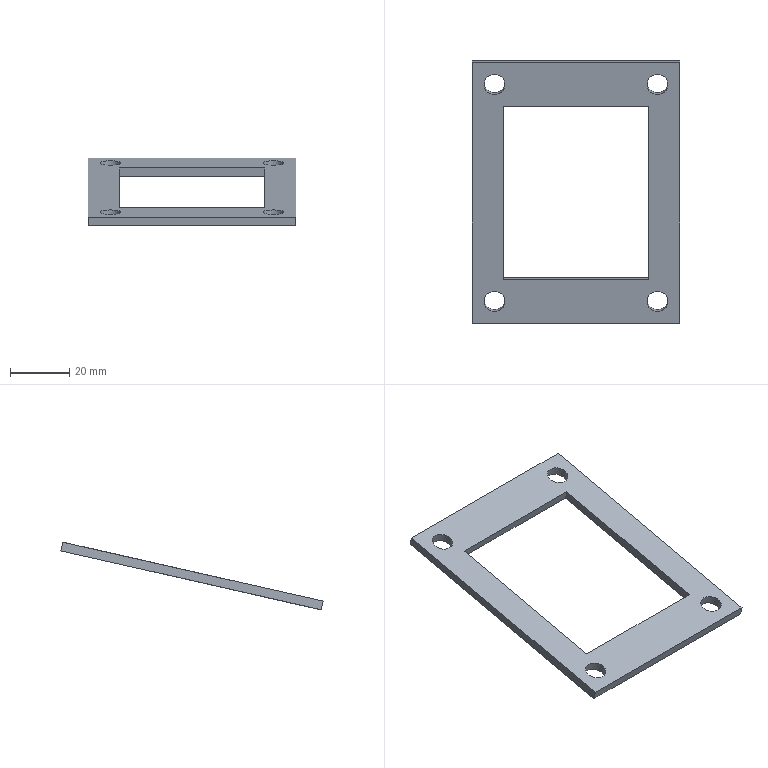Part | NX | features DATUM_CSYS 38, SIMPLE HOLE 38, SKETCH 37, EXTRACT_DATUM_AXIS 32, EXTRACT_FACE 26, HOLE PACKAGE 25, EXTRUDE 21, EXTRACT_DATUM_PLANE 14, Instance Feature 10, DRAFT 8, EXTRACT_STRING 8, BLEND 5, FSET 4, Mirror Feature 4, OFFSET_REGION 4, REPLACE_FACE 3, CPROJ 2, Pattern Feature 2, DATUM_PLANE 1, TRIM BODY 1 | 1 solid | 14 faces | box 70 x 88.433 x 22.841 mm | volume 9618 mm3 | plane 10 | cylinder 4 | commonest cylinder face diameters 7 x4
STEP:
#1=CARTESIAN_POINT('',(-35.,81.613,102.603));
#2=VERTEX_POINT('',#1);
#3=CARTESIAN_POINT('',(-35.,-6.156,82.688));
#4=VERTEX_POINT('',#3);
#5=CARTESIAN_POINT('',(-35.,81.613,102.603));
#6=DIRECTION('',(0.,-0.9752,-0.2213));
#7=VECTOR('',#6,1000.);
#8=LINE('',#5,#7);
#9=EDGE_CURVE('',#2,#4,#8,.T.);
#10=ORIENTED_EDGE('',*,*,#9,.F.);
#11=CARTESIAN_POINT('',(35.,81.613,102.603));
#12=VERTEX_POINT('',#11);
#13=CARTESIAN_POINT('',(35.,81.613,102.603));
#14=DIRECTION('',(-1.,0.,0.));
#15=VECTOR('',#14,1000.);
#16=LINE('',#13,#15);
#17=EDGE_CURVE('',#12,#2,#16,.T.);
#18=ORIENTED_EDGE('',*,*,#17,.F.);
#19=CARTESIAN_POINT('',(35.,-6.156,82.688));
#20=VERTEX_POINT('',#19);
#21=CARTESIAN_POINT('',(35.,-6.156,82.688));
#22=DIRECTION('',(0.,0.9752,0.2213));
#23=VECTOR('',#22,1000.);
#24=LINE('',#21,#23);
#25=EDGE_CURVE('',#20,#12,#24,.T.);
#26=ORIENTED_EDGE('',*,*,#25,.F.);
#27=CARTESIAN_POINT('',(-35.,-6.156,82.688));
#28=DIRECTION('',(1.,0.,0.));
#29=VECTOR('',#28,1000.);
#30=LINE('',#27,#29);
#31=EDGE_CURVE('',#4,#20,#30,.T.);
#32=ORIENTED_EDGE('',*,*,#31,.F.);
#33=EDGE_LOOP('',(#10,#18,#26,#32));
#34=FACE_BOUND('',#33,.T.);
#35=CARTESIAN_POINT('',(-27.5,4.572,85.122));
#36=VERTEX_POINT('',#35);
#37=CARTESIAN_POINT('',(-27.5,1.158,84.347));
#38=DIRECTION('',(0.,0.2213,-0.9752));
#39=DIRECTION('',(0.,0.9752,0.2213));
#40=AXIS2_PLACEMENT_3D('',#37,#38,#39);
#41=CIRCLE('',#40,3.5);
#42=EDGE_CURVE('',#36,#36,#41,.F.);
#43=ORIENTED_EDGE('',*,*,#42,.T.);
#44=EDGE_LOOP('',(#43));
#45=FACE_BOUND('',#44,.T.);
#46=CARTESIAN_POINT('',(27.5,4.572,85.122));
#47=VERTEX_POINT('',#46);
#48=CARTESIAN_POINT('',(27.5,1.158,84.347));
#49=DIRECTION('',(0.,0.2213,-0.9752));
#50=DIRECTION('',(0.,0.9752,0.2213));
#51=AXIS2_PLACEMENT_3D('',#48,#49,#50);
#52=CIRCLE('',#51,3.5);
#53=EDGE_CURVE('',#47,#47,#52,.T.);
#54=ORIENTED_EDGE('',*,*,#53,.F.);
#55=EDGE_LOOP('',(#54));
#56=FACE_BOUND('',#55,.T.);
#57=CARTESIAN_POINT('',(24.5,66.985,99.283));
#58=VERTEX_POINT('',#57);
#59=CARTESIAN_POINT('',(-24.5,66.985,99.283));
#60=VERTEX_POINT('',#59);
#61=CARTESIAN_POINT('',(-24.5,66.985,99.283));
#62=DIRECTION('',(-1.,0.,0.));
#63=VECTOR('',#62,1000.);
#64=LINE('',#61,#63);
#65=EDGE_CURVE('',#58,#60,#64,.T.);
#66=ORIENTED_EDGE('',*,*,#65,.T.);
#67=CARTESIAN_POINT('',(-24.5,8.472,86.007));
#68=VERTEX_POINT('',#67);
#69=CARTESIAN_POINT('',(-24.5,8.472,86.007));
#70=DIRECTION('',(0.,-0.9752,-0.2213));
#71=VECTOR('',#70,1000.);
#72=LINE('',#69,#71);
#73=EDGE_CURVE('',#60,#68,#72,.T.);
#74=ORIENTED_EDGE('',*,*,#73,.T.);
#75=CARTESIAN_POINT('',(24.5,8.472,86.007));
#76=VERTEX_POINT('',#75);
#77=CARTESIAN_POINT('',(24.5,8.472,86.007));
#78=DIRECTION('',(1.,0.,0.));
#79=VECTOR('',#78,1000.);
#80=LINE('',#77,#79);
#81=EDGE_CURVE('',#68,#76,#80,.T.);
#82=ORIENTED_EDGE('',*,*,#81,.T.);
#83=CARTESIAN_POINT('',(24.5,66.985,99.283));
#84=DIRECTION('',(0.,0.9752,0.2213));
#85=VECTOR('',#84,1000.);
#86=LINE('',#83,#85);
#87=EDGE_CURVE('',#76,#58,#86,.T.);
#88=ORIENTED_EDGE('',*,*,#87,.T.);
#89=EDGE_LOOP('',(#66,#74,#82,#88));
#90=FACE_BOUND('',#89,.T.);
#91=CARTESIAN_POINT('',(-27.5,77.712,101.717));
#92=VERTEX_POINT('',#91);
#93=CARTESIAN_POINT('',(-27.5,74.299,100.943));
#94=DIRECTION('',(0.,0.2213,-0.9752));
#95=DIRECTION('',(0.,0.9752,0.2213));
#96=AXIS2_PLACEMENT_3D('',#93,#94,#95);
#97=CIRCLE('',#96,3.5);
#98=EDGE_CURVE('',#92,#92,#97,.T.);
#99=ORIENTED_EDGE('',*,*,#98,.F.);
#100=EDGE_LOOP('',(#99));
#101=FACE_BOUND('',#100,.T.);
#102=CARTESIAN_POINT('',(27.5,77.712,101.717));
#103=VERTEX_POINT('',#102);
#104=CARTESIAN_POINT('',(27.5,74.299,100.943));
#105=DIRECTION('',(0.,0.2213,-0.9752));
#106=DIRECTION('',(0.,0.9752,0.2213));
#107=AXIS2_PLACEMENT_3D('',#104,#105,#106);
#108=CIRCLE('',#107,3.5);
#109=EDGE_CURVE('',#103,#103,#108,.F.);
#110=ORIENTED_EDGE('',*,*,#109,.T.);
#111=EDGE_LOOP('',(#110));
#112=FACE_BOUND('',#111,.T.);
#113=CARTESIAN_POINT('',(0.,37.729,92.645));
#114=DIRECTION('',(0.,0.2213,-0.9752));
#115=DIRECTION('',(0.,0.9752,0.2213));
#116=AXIS2_PLACEMENT_3D('',#113,#114,#115);
#117=PLANE('',#116);
#118=ADVANCED_FACE('',(#34,#45,#56,#90,#101,#112),#117,.T.);
#119=CARTESIAN_POINT('',(27.5,77.049,104.643));
#120=VERTEX_POINT('',#119);
#121=CARTESIAN_POINT('',(27.5,73.635,103.869));
#122=DIRECTION('',(0.,0.2213,-0.9752));
#123=DIRECTION('',(0.,0.9752,0.2213));
#124=AXIS2_PLACEMENT_3D('',#121,#122,#123);
#125=CIRCLE('',#124,3.5);
#126=EDGE_CURVE('',#120,#120,#125,.T.);
#127=ORIENTED_EDGE('',*,*,#126,.F.);
#128=EDGE_LOOP('',(#127));
#129=FACE_BOUND('',#128,.T.);
#130=ORIENTED_EDGE('',*,*,#109,.F.);
#131=EDGE_LOOP('',(#130));
#132=FACE_BOUND('',#131,.T.);
#133=CARTESIAN_POINT('',(27.5,73.414,104.844));
#134=DIRECTION('',(0.,0.2213,-0.9752));
#135=DIRECTION('',(0.,0.9752,0.2213));
#136=AXIS2_PLACEMENT_3D('',#133,#134,#135);
#137=CYLINDRICAL_SURFACE('',#136,3.5);
#138=ADVANCED_FACE('',(#129,#132),#137,.F.);
#139=CARTESIAN_POINT('',(-27.5,77.049,104.643));
#140=VERTEX_POINT('',#139);
#141=CARTESIAN_POINT('',(-27.5,73.635,103.869));
#142=DIRECTION('',(0.,0.2213,-0.9752));
#143=DIRECTION('',(0.,0.9752,0.2213));
#144=AXIS2_PLACEMENT_3D('',#141,#142,#143);
#145=CIRCLE('',#144,3.5);
#146=EDGE_CURVE('',#140,#140,#145,.F.);
#147=ORIENTED_EDGE('',*,*,#146,.T.);
#148=EDGE_LOOP('',(#147));
#149=FACE_BOUND('',#148,.T.);
#150=ORIENTED_EDGE('',*,*,#98,.T.);
#151=EDGE_LOOP('',(#150));
#152=FACE_BOUND('',#151,.T.);
#153=CARTESIAN_POINT('',(-27.5,73.414,104.844));
#154=DIRECTION('',(0.,0.2213,-0.9752));
#155=DIRECTION('',(0.,0.9752,0.2213));
#156=AXIS2_PLACEMENT_3D('',#153,#154,#155);
#157=CYLINDRICAL_SURFACE('',#156,3.5);
#158=ADVANCED_FACE('',(#149,#152),#157,.F.);
#159=ORIENTED_EDGE('',*,*,#73,.F.);
#160=CARTESIAN_POINT('',(-24.5,66.321,102.209));
#161=VERTEX_POINT('',#160);
#162=CARTESIAN_POINT('',(-24.5,66.1,103.184));
#163=DIRECTION('',(0.,0.2213,-0.9752));
#164=VECTOR('',#163,1000.);
#165=LINE('',#162,#164);
#166=EDGE_CURVE('',#161,#60,#165,.T.);
#167=ORIENTED_EDGE('',*,*,#166,.F.);
#168=CARTESIAN_POINT('',(-24.5,7.809,88.932));
#169=VERTEX_POINT('',#168);
#170=CARTESIAN_POINT('',(-24.5,73.635,103.869));
#171=DIRECTION('',(0.,0.9752,0.2213));
#172=VECTOR('',#171,1000.);
#173=LINE('',#170,#172);
#174=EDGE_CURVE('',#169,#161,#173,.T.);
#175=ORIENTED_EDGE('',*,*,#174,.F.);
#176=CARTESIAN_POINT('',(-24.5,7.587,89.908));
#177=DIRECTION('',(0.,0.2213,-0.9752));
#178=VECTOR('',#177,1000.);
#179=LINE('',#176,#178);
#180=EDGE_CURVE('',#169,#68,#179,.T.);
#181=ORIENTED_EDGE('',*,*,#180,.T.);
#182=EDGE_LOOP('',(#159,#167,#175,#181));
#183=FACE_BOUND('',#182,.T.);
#184=CARTESIAN_POINT('',(-24.5,7.587,89.908));
#185=DIRECTION('',(-1.,0.,0.));
#186=DIRECTION('',(0.,0.,1.));
#187=AXIS2_PLACEMENT_3D('',#184,#185,#186);
#188=PLANE('',#187);
#189=ADVANCED_FACE('',(#183),#188,.F.);
#190=ORIENTED_EDGE('',*,*,#65,.F.);
#191=CARTESIAN_POINT('',(24.5,66.321,102.209));
#192=VERTEX_POINT('',#191);
#193=CARTESIAN_POINT('',(24.5,66.1,103.184));
#194=DIRECTION('',(0.,0.2213,-0.9752));
#195=VECTOR('',#194,1000.);
#196=LINE('',#193,#195);
#197=EDGE_CURVE('',#192,#58,#196,.T.);
#198=ORIENTED_EDGE('',*,*,#197,.F.);
#199=CARTESIAN_POINT('',(27.5,66.321,102.209));
#200=DIRECTION('',(1.,0.,0.));
#201=VECTOR('',#200,1000.);
#202=LINE('',#199,#201);
#203=EDGE_CURVE('',#161,#192,#202,.T.);
#204=ORIENTED_EDGE('',*,*,#203,.F.);
#205=ORIENTED_EDGE('',*,*,#166,.T.);
#206=EDGE_LOOP('',(#190,#198,#204,#205));
#207=FACE_BOUND('',#206,.T.);
#208=CARTESIAN_POINT('',(-24.5,66.1,103.184));
#209=DIRECTION('',(0.,0.9752,0.2213));
#210=DIRECTION('',(0.,-0.2213,0.9752));
#211=AXIS2_PLACEMENT_3D('',#208,#209,#210);
#212=PLANE('',#211);
#213=ADVANCED_FACE('',(#207),#212,.F.);
#214=ORIENTED_EDGE('',*,*,#87,.F.);
#215=CARTESIAN_POINT('',(24.5,7.809,88.932));
#216=VERTEX_POINT('',#215);
#217=CARTESIAN_POINT('',(24.5,7.587,89.908));
#218=DIRECTION('',(0.,0.2213,-0.9752));
#219=VECTOR('',#218,1000.);
#220=LINE('',#217,#219);
#221=EDGE_CURVE('',#216,#76,#220,.T.);
#222=ORIENTED_EDGE('',*,*,#221,.F.);
#223=CARTESIAN_POINT('',(24.5,73.635,103.869));
#224=DIRECTION('',(0.,-0.9752,-0.2213));
#225=VECTOR('',#224,1000.);
#226=LINE('',#223,#225);
#227=EDGE_CURVE('',#192,#216,#226,.T.);
#228=ORIENTED_EDGE('',*,*,#227,.F.);
#229=ORIENTED_EDGE('',*,*,#197,.T.);
#230=EDGE_LOOP('',(#214,#222,#228,#229));
#231=FACE_BOUND('',#230,.T.);
#232=CARTESIAN_POINT('',(24.5,66.1,103.184));
#233=DIRECTION('',(1.,0.,0.));
#234=DIRECTION('',(0.,0.,-1.));
#235=AXIS2_PLACEMENT_3D('',#232,#233,#234);
#236=PLANE('',#235);
#237=ADVANCED_FACE('',(#231),#236,.F.);
#238=CARTESIAN_POINT('',(-27.5,3.908,88.047));
#239=VERTEX_POINT('',#238);
#240=CARTESIAN_POINT('',(-27.5,0.4945,87.273));
#241=DIRECTION('',(0.,0.2213,-0.9752));
#242=DIRECTION('',(0.,0.9752,0.2213));
#243=AXIS2_PLACEMENT_3D('',#240,#241,#242);
#244=CIRCLE('',#243,3.5);
#245=EDGE_CURVE('',#239,#239,#244,.T.);
#246=ORIENTED_EDGE('',*,*,#245,.F.);
#247=EDGE_LOOP('',(#246));
#248=FACE_BOUND('',#247,.T.);
#249=ORIENTED_EDGE('',*,*,#42,.F.);
#250=EDGE_LOOP('',(#249));
#251=FACE_BOUND('',#250,.T.);
#252=CARTESIAN_POINT('',(-27.5,0.2732,88.248));
#253=DIRECTION('',(0.,0.2213,-0.9752));
#254=DIRECTION('',(0.,0.9752,0.2213));
#255=AXIS2_PLACEMENT_3D('',#252,#253,#254);
#256=CYLINDRICAL_SURFACE('',#255,3.5);
#257=ADVANCED_FACE('',(#248,#251),#256,.F.);
#258=CARTESIAN_POINT('',(27.5,3.908,88.047));
#259=VERTEX_POINT('',#258);
#260=CARTESIAN_POINT('',(27.5,0.4945,87.273));
#261=DIRECTION('',(0.,0.2213,-0.9752));
#262=DIRECTION('',(0.,0.9752,0.2213));
#263=AXIS2_PLACEMENT_3D('',#260,#261,#262);
#264=CIRCLE('',#263,3.5);
#265=EDGE_CURVE('',#259,#259,#264,.F.);
#266=ORIENTED_EDGE('',*,*,#265,.T.);
#267=EDGE_LOOP('',(#266));
#268=FACE_BOUND('',#267,.T.);
#269=ORIENTED_EDGE('',*,*,#53,.T.);
#270=EDGE_LOOP('',(#269));
#271=FACE_BOUND('',#270,.T.);
#272=CARTESIAN_POINT('',(27.5,0.2732,88.248));
#273=DIRECTION('',(0.,0.2213,-0.9752));
#274=DIRECTION('',(0.,0.9752,0.2213));
#275=AXIS2_PLACEMENT_3D('',#272,#273,#274);
#276=CYLINDRICAL_SURFACE('',#275,3.5);
#277=ADVANCED_FACE('',(#268,#271),#276,.F.);
#278=ORIENTED_EDGE('',*,*,#81,.F.);
#279=ORIENTED_EDGE('',*,*,#180,.F.);
#280=CARTESIAN_POINT('',(27.5,7.809,88.932));
#281=DIRECTION('',(-1.,0.,0.));
#282=VECTOR('',#281,1000.);
#283=LINE('',#280,#282);
#284=EDGE_CURVE('',#216,#169,#283,.T.);
#285=ORIENTED_EDGE('',*,*,#284,.F.);
#286=ORIENTED_EDGE('',*,*,#221,.T.);
#287=EDGE_LOOP('',(#278,#279,#285,#286));
#288=FACE_BOUND('',#287,.T.);
#289=CARTESIAN_POINT('',(24.5,7.587,89.908));
#290=DIRECTION('',(0.,-0.9752,-0.2213));
#291=DIRECTION('',(0.,0.2213,-0.9752));
#292=AXIS2_PLACEMENT_3D('',#289,#290,#291);
#293=PLANE('',#292);
#294=ADVANCED_FACE('',(#288),#293,.F.);
#295=ORIENTED_EDGE('',*,*,#9,.T.);
#296=CARTESIAN_POINT('',(-35.,-6.82,85.613));
#297=VERTEX_POINT('',#296);
#298=CARTESIAN_POINT('',(-35.,-7.041,86.588));
#299=DIRECTION('',(0.,0.2213,-0.9752));
#300=VECTOR('',#299,1000.);
#301=LINE('',#298,#300);
#302=EDGE_CURVE('',#297,#4,#301,.T.);
#303=ORIENTED_EDGE('',*,*,#302,.F.);
#304=CARTESIAN_POINT('',(-35.,80.949,105.528));
#305=VERTEX_POINT('',#304);
#306=CARTESIAN_POINT('',(-35.,73.635,103.869));
#307=DIRECTION('',(0.,-0.9752,-0.2213));
#308=VECTOR('',#307,1000.);
#309=LINE('',#306,#308);
#310=EDGE_CURVE('',#305,#297,#309,.T.);
#311=ORIENTED_EDGE('',*,*,#310,.F.);
#312=CARTESIAN_POINT('',(-35.,80.728,106.503));
#313=DIRECTION('',(0.,0.2213,-0.9752));
#314=VECTOR('',#313,1000.);
#315=LINE('',#312,#314);
#316=EDGE_CURVE('',#305,#2,#315,.T.);
#317=ORIENTED_EDGE('',*,*,#316,.T.);
#318=EDGE_LOOP('',(#295,#303,#311,#317));
#319=FACE_BOUND('',#318,.T.);
#320=CARTESIAN_POINT('',(-35.,80.728,106.503));
#321=DIRECTION('',(1.,0.,0.));
#322=DIRECTION('',(0.,0.,-1.));
#323=AXIS2_PLACEMENT_3D('',#320,#321,#322);
#324=PLANE('',#323);
#325=ADVANCED_FACE('',(#319),#324,.F.);
#326=ORIENTED_EDGE('',*,*,#31,.T.);
#327=CARTESIAN_POINT('',(35.,-6.82,85.613));
#328=VERTEX_POINT('',#327);
#329=CARTESIAN_POINT('',(35.,-7.041,86.588));
#330=DIRECTION('',(0.,0.2213,-0.9752));
#331=VECTOR('',#330,1000.);
#332=LINE('',#329,#331);
#333=EDGE_CURVE('',#328,#20,#332,.T.);
#334=ORIENTED_EDGE('',*,*,#333,.F.);
#335=CARTESIAN_POINT('',(27.5,-6.82,85.613));
#336=DIRECTION('',(1.,0.,0.));
#337=VECTOR('',#336,1000.);
#338=LINE('',#335,#337);
#339=EDGE_CURVE('',#297,#328,#338,.T.);
#340=ORIENTED_EDGE('',*,*,#339,.F.);
#341=ORIENTED_EDGE('',*,*,#302,.T.);
#342=EDGE_LOOP('',(#326,#334,#340,#341));
#343=FACE_BOUND('',#342,.T.);
#344=CARTESIAN_POINT('',(-35.,-7.041,86.588));
#345=DIRECTION('',(0.,0.9752,0.2213));
#346=DIRECTION('',(0.,-0.2213,0.9752));
#347=AXIS2_PLACEMENT_3D('',#344,#345,#346);
#348=PLANE('',#347);
#349=ADVANCED_FACE('',(#343),#348,.F.);
#350=ORIENTED_EDGE('',*,*,#25,.T.);
#351=CARTESIAN_POINT('',(35.,80.949,105.528));
#352=VERTEX_POINT('',#351);
#353=CARTESIAN_POINT('',(35.,80.728,106.503));
#354=DIRECTION('',(0.,0.2213,-0.9752));
#355=VECTOR('',#354,1000.);
#356=LINE('',#353,#355);
#357=EDGE_CURVE('',#352,#12,#356,.T.);
#358=ORIENTED_EDGE('',*,*,#357,.F.);
#359=CARTESIAN_POINT('',(35.,73.635,103.869));
#360=DIRECTION('',(0.,0.9752,0.2213));
#361=VECTOR('',#360,1000.);
#362=LINE('',#359,#361);
#363=EDGE_CURVE('',#328,#352,#362,.T.);
#364=ORIENTED_EDGE('',*,*,#363,.F.);
#365=ORIENTED_EDGE('',*,*,#333,.T.);
#366=EDGE_LOOP('',(#350,#358,#364,#365));
#367=FACE_BOUND('',#366,.T.);
#368=CARTESIAN_POINT('',(35.,-7.041,86.588));
#369=DIRECTION('',(-1.,0.,0.));
#370=DIRECTION('',(0.,0.,1.));
#371=AXIS2_PLACEMENT_3D('',#368,#369,#370);
#372=PLANE('',#371);
#373=ADVANCED_FACE('',(#367),#372,.F.);
#374=ORIENTED_EDGE('',*,*,#17,.T.);
#375=ORIENTED_EDGE('',*,*,#316,.F.);
#376=CARTESIAN_POINT('',(27.5,80.949,105.528));
#377=DIRECTION('',(-1.,0.,0.));
#378=VECTOR('',#377,1000.);
#379=LINE('',#376,#378);
#380=EDGE_CURVE('',#352,#305,#379,.T.);
#381=ORIENTED_EDGE('',*,*,#380,.F.);
#382=ORIENTED_EDGE('',*,*,#357,.T.);
#383=EDGE_LOOP('',(#374,#375,#381,#382));
#384=FACE_BOUND('',#383,.T.);
#385=CARTESIAN_POINT('',(35.,80.728,106.503));
#386=DIRECTION('',(0.,-0.9752,-0.2213));
#387=DIRECTION('',(0.,0.2213,-0.9752));
#388=AXIS2_PLACEMENT_3D('',#385,#386,#387);
#389=PLANE('',#388);
#390=ADVANCED_FACE('',(#384),#389,.F.);
#391=ORIENTED_EDGE('',*,*,#310,.T.);
#392=ORIENTED_EDGE('',*,*,#339,.T.);
#393=ORIENTED_EDGE('',*,*,#363,.T.);
#394=ORIENTED_EDGE('',*,*,#380,.T.);
#395=EDGE_LOOP('',(#391,#392,#393,#394));
#396=FACE_BOUND('',#395,.T.);
#397=ORIENTED_EDGE('',*,*,#126,.T.);
#398=EDGE_LOOP('',(#397));
#399=FACE_BOUND('',#398,.T.);
#400=ORIENTED_EDGE('',*,*,#265,.F.);
#401=EDGE_LOOP('',(#400));
#402=FACE_BOUND('',#401,.T.);
#403=ORIENTED_EDGE('',*,*,#146,.F.);
#404=EDGE_LOOP('',(#403));
#405=FACE_BOUND('',#404,.T.);
#406=ORIENTED_EDGE('',*,*,#245,.T.);
#407=EDGE_LOOP('',(#406));
#408=FACE_BOUND('',#407,.T.);
#409=ORIENTED_EDGE('',*,*,#174,.T.);
#410=ORIENTED_EDGE('',*,*,#203,.T.);
#411=ORIENTED_EDGE('',*,*,#227,.T.);
#412=ORIENTED_EDGE('',*,*,#284,.T.);
#413=EDGE_LOOP('',(#409,#410,#411,#412));
#414=FACE_BOUND('',#413,.T.);
#415=CARTESIAN_POINT('',(27.5,73.635,103.869));
#416=DIRECTION('',(0.,0.2213,-0.9752));
#417=DIRECTION('',(0.,0.9752,0.2213));
#418=AXIS2_PLACEMENT_3D('',#415,#416,#417);
#419=PLANE('',#418);
#420=ADVANCED_FACE('',(#396,#399,#402,#405,#408,#414),#419,.F.);
#421=CLOSED_SHELL('',(#118,#138,#158,#189,#213,#237,#257,#277,#294,#325,#349,#373,#390,#420));
#422=MANIFOLD_SOLID_BREP('',#421);
#423=(LENGTH_UNIT()NAMED_UNIT(*)SI_UNIT(.MILLI.,.METRE.));
#424=UNCERTAINTY_MEASURE_WITH_UNIT(LENGTH_MEASURE(0.00001),#423,'','');
#425=(NAMED_UNIT(*)PLANE_ANGLE_UNIT()SI_UNIT($,.RADIAN.));
#426=(NAMED_UNIT(*)SI_UNIT($,.STERADIAN.)SOLID_ANGLE_UNIT());
#427=(GEOMETRIC_REPRESENTATION_CONTEXT(3)GLOBAL_UNCERTAINTY_ASSIGNED_CONTEXT((#424))GLOBAL_UNIT_ASSIGNED_CONTEXT((#423,#425,#426))REPRESENTATION_CONTEXT('',''));
#428=ADVANCED_BREP_SHAPE_REPRESENTATION('',(#422),#427);